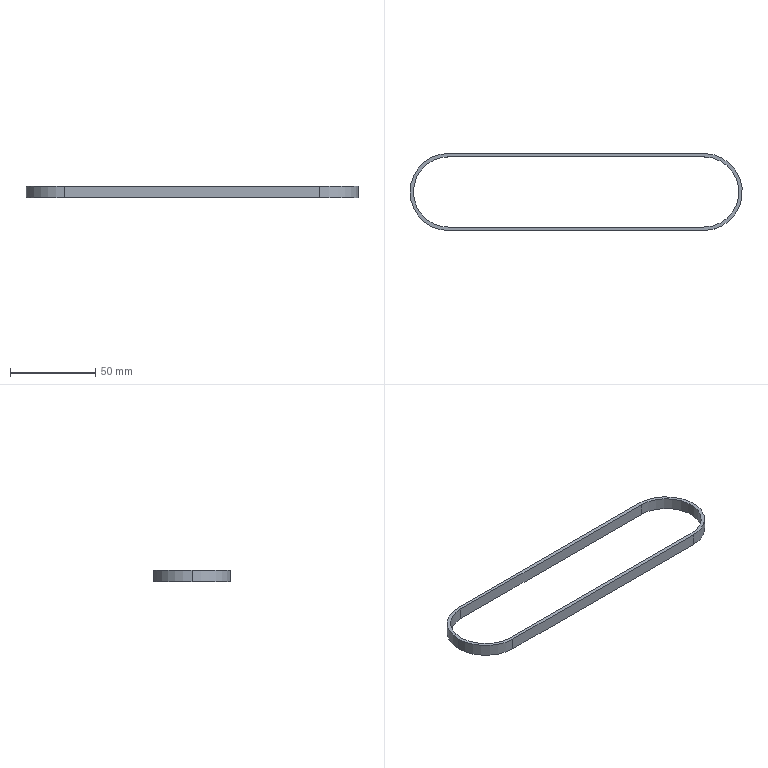Part | SolidWorks | features ExtruThin 1 | 1 solid | 12 faces | box 195.3 x 45.3 x 7 mm | volume 6104 mm3 | cylinder 6 | plane 6 | commonest cylinder face diameters 41.3 x3 45.3 x3
STEP:
#1=CARTESIAN_POINT('',(0.,20.65,3.5));
#2=VERTEX_POINT('',#1);
#3=CARTESIAN_POINT('',(-20.65,0.,3.5));
#4=VERTEX_POINT('',#3);
#5=CARTESIAN_POINT('',(0.,0.,3.5));
#6=DIRECTION('',(0.,0.,1.));
#7=DIRECTION('',(1.,0.,0.));
#8=AXIS2_PLACEMENT_3D('',#5,#6,#7);
#9=CIRCLE('',#8,20.65);
#10=EDGE_CURVE('',#2,#4,#9,.T.);
#11=ORIENTED_EDGE('',*,*,#10,.T.);
#12=CARTESIAN_POINT('',(-20.65,0.,-3.5));
#13=VERTEX_POINT('',#12);
#14=CARTESIAN_POINT('',(-20.65,0.,3.5));
#15=DIRECTION('',(0.,0.,-1.));
#16=VECTOR('',#15,1000.);
#17=LINE('',#14,#16);
#18=EDGE_CURVE('',#4,#13,#17,.T.);
#19=ORIENTED_EDGE('',*,*,#18,.T.);
#20=CARTESIAN_POINT('',(0.,20.65,-3.5));
#21=VERTEX_POINT('',#20);
#22=CARTESIAN_POINT('',(0.,0.,-3.5));
#23=DIRECTION('',(0.,0.,1.));
#24=DIRECTION('',(1.,0.,0.));
#25=AXIS2_PLACEMENT_3D('',#22,#23,#24);
#26=CIRCLE('',#25,20.65);
#27=EDGE_CURVE('',#21,#13,#26,.T.);
#28=ORIENTED_EDGE('',*,*,#27,.F.);
#29=CARTESIAN_POINT('',(0.,20.65,3.5));
#30=DIRECTION('',(0.,0.,-1.));
#31=VECTOR('',#30,1000.);
#32=LINE('',#29,#31);
#33=EDGE_CURVE('',#2,#21,#32,.T.);
#34=ORIENTED_EDGE('',*,*,#33,.F.);
#35=EDGE_LOOP('',(#11,#19,#28,#34));
#36=FACE_OUTER_BOUND('',#35,.T.);
#37=CARTESIAN_POINT('',(0.,0.,3.5));
#38=DIRECTION('',(0.,0.,-1.));
#39=DIRECTION('',(-1.,0.,0.));
#40=AXIS2_PLACEMENT_3D('',#37,#38,#39);
#41=CYLINDRICAL_SURFACE('',#40,20.65);
#42=ADVANCED_FACE('',(#36),#41,.F.);
#43=CARTESIAN_POINT('',(-22.65,0.,3.5));
#44=VERTEX_POINT('',#43);
#45=CARTESIAN_POINT('',(0.,-22.65,3.5));
#46=VERTEX_POINT('',#45);
#47=CARTESIAN_POINT('',(0.,0.,3.5));
#48=DIRECTION('',(0.,0.,1.));
#49=DIRECTION('',(1.,0.,0.));
#50=AXIS2_PLACEMENT_3D('',#47,#48,#49);
#51=CIRCLE('',#50,22.65);
#52=EDGE_CURVE('',#44,#46,#51,.T.);
#53=ORIENTED_EDGE('',*,*,#52,.F.);
#54=CARTESIAN_POINT('',(-22.65,0.,-3.5));
#55=VERTEX_POINT('',#54);
#56=CARTESIAN_POINT('',(-22.65,0.,3.5));
#57=DIRECTION('',(0.,0.,-1.));
#58=VECTOR('',#57,1000.);
#59=LINE('',#56,#58);
#60=EDGE_CURVE('',#44,#55,#59,.T.);
#61=ORIENTED_EDGE('',*,*,#60,.T.);
#62=CARTESIAN_POINT('',(0.,-22.65,-3.5));
#63=VERTEX_POINT('',#62);
#64=CARTESIAN_POINT('',(0.,0.,-3.5));
#65=DIRECTION('',(0.,0.,1.));
#66=DIRECTION('',(1.,0.,0.));
#67=AXIS2_PLACEMENT_3D('',#64,#65,#66);
#68=CIRCLE('',#67,22.65);
#69=EDGE_CURVE('',#55,#63,#68,.T.);
#70=ORIENTED_EDGE('',*,*,#69,.T.);
#71=CARTESIAN_POINT('',(0.,-22.65,3.5));
#72=DIRECTION('',(0.,0.,-1.));
#73=VECTOR('',#72,1000.);
#74=LINE('',#71,#73);
#75=EDGE_CURVE('',#46,#63,#74,.T.);
#76=ORIENTED_EDGE('',*,*,#75,.F.);
#77=EDGE_LOOP('',(#53,#61,#70,#76));
#78=FACE_OUTER_BOUND('',#77,.T.);
#79=CARTESIAN_POINT('',(0.,0.,3.5));
#80=DIRECTION('',(0.,0.,-1.));
#81=DIRECTION('',(-1.,0.,0.));
#82=AXIS2_PLACEMENT_3D('',#79,#80,#81);
#83=CYLINDRICAL_SURFACE('',#82,22.65);
#84=ADVANCED_FACE('',(#78),#83,.T.);
#85=CARTESIAN_POINT('',(0.,22.65,3.5));
#86=VERTEX_POINT('',#85);
#87=CARTESIAN_POINT('',(0.,0.,3.5));
#88=DIRECTION('',(0.,0.,1.));
#89=DIRECTION('',(1.,0.,0.));
#90=AXIS2_PLACEMENT_3D('',#87,#88,#89);
#91=CIRCLE('',#90,22.65);
#92=EDGE_CURVE('',#86,#44,#91,.T.);
#93=ORIENTED_EDGE('',*,*,#92,.T.);
#94=ORIENTED_EDGE('',*,*,#52,.T.);
#95=CARTESIAN_POINT('',(150.,-22.65,3.5));
#96=VERTEX_POINT('',#95);
#97=CARTESIAN_POINT('',(0.,-22.65,3.5));
#98=DIRECTION('',(1.,0.,0.));
#99=VECTOR('',#98,1000.);
#100=LINE('',#97,#99);
#101=EDGE_CURVE('',#46,#96,#100,.T.);
#102=ORIENTED_EDGE('',*,*,#101,.T.);
#103=CARTESIAN_POINT('',(150.,22.65,3.5));
#104=VERTEX_POINT('',#103);
#105=CARTESIAN_POINT('',(150.,0.,3.5));
#106=DIRECTION('',(0.,0.,1.));
#107=DIRECTION('',(1.,0.,0.));
#108=AXIS2_PLACEMENT_3D('',#105,#106,#107);
#109=CIRCLE('',#108,22.65);
#110=EDGE_CURVE('',#96,#104,#109,.T.);
#111=ORIENTED_EDGE('',*,*,#110,.T.);
#112=CARTESIAN_POINT('',(0.,22.65,3.5));
#113=DIRECTION('',(-1.,0.,0.));
#114=VECTOR('',#113,1000.);
#115=LINE('',#112,#114);
#116=EDGE_CURVE('',#104,#86,#115,.T.);
#117=ORIENTED_EDGE('',*,*,#116,.T.);
#118=EDGE_LOOP('',(#93,#94,#102,#111,#117));
#119=FACE_OUTER_BOUND('',#118,.T.);
#120=CARTESIAN_POINT('',(0.,-20.65,3.5));
#121=VERTEX_POINT('',#120);
#122=CARTESIAN_POINT('',(150.,-20.65,3.5));
#123=VERTEX_POINT('',#122);
#124=CARTESIAN_POINT('',(0.,-20.65,3.5));
#125=DIRECTION('',(1.,0.,0.));
#126=VECTOR('',#125,1000.);
#127=LINE('',#124,#126);
#128=EDGE_CURVE('',#121,#123,#127,.T.);
#129=ORIENTED_EDGE('',*,*,#128,.F.);
#130=CARTESIAN_POINT('',(0.,0.,3.5));
#131=DIRECTION('',(0.,0.,1.));
#132=DIRECTION('',(1.,0.,0.));
#133=AXIS2_PLACEMENT_3D('',#130,#131,#132);
#134=CIRCLE('',#133,20.65);
#135=EDGE_CURVE('',#4,#121,#134,.T.);
#136=ORIENTED_EDGE('',*,*,#135,.F.);
#137=ORIENTED_EDGE('',*,*,#10,.F.);
#138=CARTESIAN_POINT('',(150.,20.65,3.5));
#139=VERTEX_POINT('',#138);
#140=CARTESIAN_POINT('',(0.,20.65,3.5));
#141=DIRECTION('',(-1.,0.,0.));
#142=VECTOR('',#141,1000.);
#143=LINE('',#140,#142);
#144=EDGE_CURVE('',#139,#2,#143,.T.);
#145=ORIENTED_EDGE('',*,*,#144,.F.);
#146=CARTESIAN_POINT('',(150.,0.,3.5));
#147=DIRECTION('',(0.,0.,1.));
#148=DIRECTION('',(1.,0.,0.));
#149=AXIS2_PLACEMENT_3D('',#146,#147,#148);
#150=CIRCLE('',#149,20.65);
#151=EDGE_CURVE('',#123,#139,#150,.T.);
#152=ORIENTED_EDGE('',*,*,#151,.F.);
#153=EDGE_LOOP('',(#129,#136,#137,#145,#152));
#154=FACE_BOUND('',#153,.T.);
#155=CARTESIAN_POINT('',(0.,0.,3.5));
#156=DIRECTION('',(0.,0.,1.));
#157=DIRECTION('',(1.,0.,0.));
#158=AXIS2_PLACEMENT_3D('',#155,#156,#157);
#159=PLANE('',#158);
#160=ADVANCED_FACE('',(#119,#154),#159,.T.);
#161=CARTESIAN_POINT('',(0.,22.65,-3.5));
#162=VERTEX_POINT('',#161);
#163=CARTESIAN_POINT('',(0.,0.,-3.5));
#164=DIRECTION('',(0.,0.,1.));
#165=DIRECTION('',(1.,0.,0.));
#166=AXIS2_PLACEMENT_3D('',#163,#164,#165);
#167=CIRCLE('',#166,22.65);
#168=EDGE_CURVE('',#162,#55,#167,.T.);
#169=ORIENTED_EDGE('',*,*,#168,.F.);
#170=CARTESIAN_POINT('',(150.,22.65,-3.5));
#171=VERTEX_POINT('',#170);
#172=CARTESIAN_POINT('',(0.,22.65,-3.5));
#173=DIRECTION('',(-1.,0.,0.));
#174=VECTOR('',#173,1000.);
#175=LINE('',#172,#174);
#176=EDGE_CURVE('',#171,#162,#175,.T.);
#177=ORIENTED_EDGE('',*,*,#176,.F.);
#178=CARTESIAN_POINT('',(150.,-22.65,-3.5));
#179=VERTEX_POINT('',#178);
#180=CARTESIAN_POINT('',(150.,0.,-3.5));
#181=DIRECTION('',(0.,0.,1.));
#182=DIRECTION('',(1.,0.,0.));
#183=AXIS2_PLACEMENT_3D('',#180,#181,#182);
#184=CIRCLE('',#183,22.65);
#185=EDGE_CURVE('',#179,#171,#184,.T.);
#186=ORIENTED_EDGE('',*,*,#185,.F.);
#187=CARTESIAN_POINT('',(0.,-22.65,-3.5));
#188=DIRECTION('',(1.,0.,0.));
#189=VECTOR('',#188,1000.);
#190=LINE('',#187,#189);
#191=EDGE_CURVE('',#63,#179,#190,.T.);
#192=ORIENTED_EDGE('',*,*,#191,.F.);
#193=ORIENTED_EDGE('',*,*,#69,.F.);
#194=EDGE_LOOP('',(#169,#177,#186,#192,#193));
#195=FACE_OUTER_BOUND('',#194,.T.);
#196=ORIENTED_EDGE('',*,*,#27,.T.);
#197=CARTESIAN_POINT('',(0.,-20.65,-3.5));
#198=VERTEX_POINT('',#197);
#199=CARTESIAN_POINT('',(0.,0.,-3.5));
#200=DIRECTION('',(0.,0.,1.));
#201=DIRECTION('',(1.,0.,0.));
#202=AXIS2_PLACEMENT_3D('',#199,#200,#201);
#203=CIRCLE('',#202,20.65);
#204=EDGE_CURVE('',#13,#198,#203,.T.);
#205=ORIENTED_EDGE('',*,*,#204,.T.);
#206=CARTESIAN_POINT('',(150.,-20.65,-3.5));
#207=VERTEX_POINT('',#206);
#208=CARTESIAN_POINT('',(0.,-20.65,-3.5));
#209=DIRECTION('',(1.,0.,0.));
#210=VECTOR('',#209,1000.);
#211=LINE('',#208,#210);
#212=EDGE_CURVE('',#198,#207,#211,.T.);
#213=ORIENTED_EDGE('',*,*,#212,.T.);
#214=CARTESIAN_POINT('',(150.,20.65,-3.5));
#215=VERTEX_POINT('',#214);
#216=CARTESIAN_POINT('',(150.,0.,-3.5));
#217=DIRECTION('',(0.,0.,1.));
#218=DIRECTION('',(1.,0.,0.));
#219=AXIS2_PLACEMENT_3D('',#216,#217,#218);
#220=CIRCLE('',#219,20.65);
#221=EDGE_CURVE('',#207,#215,#220,.T.);
#222=ORIENTED_EDGE('',*,*,#221,.T.);
#223=CARTESIAN_POINT('',(0.,20.65,-3.5));
#224=DIRECTION('',(-1.,0.,0.));
#225=VECTOR('',#224,1000.);
#226=LINE('',#223,#225);
#227=EDGE_CURVE('',#215,#21,#226,.T.);
#228=ORIENTED_EDGE('',*,*,#227,.T.);
#229=EDGE_LOOP('',(#196,#205,#213,#222,#228));
#230=FACE_BOUND('',#229,.T.);
#231=CARTESIAN_POINT('',(0.,0.,-3.5));
#232=DIRECTION('',(0.,0.,1.));
#233=DIRECTION('',(1.,0.,0.));
#234=AXIS2_PLACEMENT_3D('',#231,#232,#233);
#235=PLANE('',#234);
#236=ADVANCED_FACE('',(#195,#230),#235,.F.);
#237=ORIENTED_EDGE('',*,*,#60,.F.);
#238=ORIENTED_EDGE('',*,*,#92,.F.);
#239=CARTESIAN_POINT('',(0.,22.65,3.5));
#240=DIRECTION('',(0.,0.,-1.));
#241=VECTOR('',#240,1000.);
#242=LINE('',#239,#241);
#243=EDGE_CURVE('',#86,#162,#242,.T.);
#244=ORIENTED_EDGE('',*,*,#243,.T.);
#245=ORIENTED_EDGE('',*,*,#168,.T.);
#246=EDGE_LOOP('',(#237,#238,#244,#245));
#247=FACE_OUTER_BOUND('',#246,.T.);
#248=CARTESIAN_POINT('',(0.,0.,3.5));
#249=DIRECTION('',(0.,0.,-1.));
#250=DIRECTION('',(-1.,0.,0.));
#251=AXIS2_PLACEMENT_3D('',#248,#249,#250);
#252=CYLINDRICAL_SURFACE('',#251,22.65);
#253=ADVANCED_FACE('',(#247),#252,.T.);
#254=ORIENTED_EDGE('',*,*,#191,.T.);
#255=CARTESIAN_POINT('',(150.,-22.65,3.5));
#256=DIRECTION('',(0.,0.,-1.));
#257=VECTOR('',#256,1000.);
#258=LINE('',#255,#257);
#259=EDGE_CURVE('',#96,#179,#258,.T.);
#260=ORIENTED_EDGE('',*,*,#259,.F.);
#261=ORIENTED_EDGE('',*,*,#101,.F.);
#262=ORIENTED_EDGE('',*,*,#75,.T.);
#263=EDGE_LOOP('',(#254,#260,#261,#262));
#264=FACE_OUTER_BOUND('',#263,.T.);
#265=CARTESIAN_POINT('',(0.,-22.65,3.5));
#266=DIRECTION('',(0.,1.,0.));
#267=DIRECTION('',(0.,0.,1.));
#268=AXIS2_PLACEMENT_3D('',#265,#266,#267);
#269=PLANE('',#268);
#270=ADVANCED_FACE('',(#264),#269,.F.);
#271=ORIENTED_EDGE('',*,*,#185,.T.);
#272=CARTESIAN_POINT('',(150.,22.65,3.5));
#273=DIRECTION('',(0.,0.,-1.));
#274=VECTOR('',#273,1000.);
#275=LINE('',#272,#274);
#276=EDGE_CURVE('',#104,#171,#275,.T.);
#277=ORIENTED_EDGE('',*,*,#276,.F.);
#278=ORIENTED_EDGE('',*,*,#110,.F.);
#279=ORIENTED_EDGE('',*,*,#259,.T.);
#280=EDGE_LOOP('',(#271,#277,#278,#279));
#281=FACE_OUTER_BOUND('',#280,.T.);
#282=CARTESIAN_POINT('',(150.,0.,3.5));
#283=DIRECTION('',(0.,0.,-1.));
#284=DIRECTION('',(-1.,0.,0.));
#285=AXIS2_PLACEMENT_3D('',#282,#283,#284);
#286=CYLINDRICAL_SURFACE('',#285,22.65);
#287=ADVANCED_FACE('',(#281),#286,.T.);
#288=ORIENTED_EDGE('',*,*,#176,.T.);
#289=ORIENTED_EDGE('',*,*,#243,.F.);
#290=ORIENTED_EDGE('',*,*,#116,.F.);
#291=ORIENTED_EDGE('',*,*,#276,.T.);
#292=EDGE_LOOP('',(#288,#289,#290,#291));
#293=FACE_OUTER_BOUND('',#292,.T.);
#294=CARTESIAN_POINT('',(0.,22.65,3.5));
#295=DIRECTION('',(0.,-1.,0.));
#296=DIRECTION('',(0.,0.,-1.));
#297=AXIS2_PLACEMENT_3D('',#294,#295,#296);
#298=PLANE('',#297);
#299=ADVANCED_FACE('',(#293),#298,.F.);
#300=ORIENTED_EDGE('',*,*,#18,.F.);
#301=ORIENTED_EDGE('',*,*,#135,.T.);
#302=CARTESIAN_POINT('',(0.,-20.65,3.5));
#303=DIRECTION('',(0.,0.,-1.));
#304=VECTOR('',#303,1000.);
#305=LINE('',#302,#304);
#306=EDGE_CURVE('',#121,#198,#305,.T.);
#307=ORIENTED_EDGE('',*,*,#306,.T.);
#308=ORIENTED_EDGE('',*,*,#204,.F.);
#309=EDGE_LOOP('',(#300,#301,#307,#308));
#310=FACE_OUTER_BOUND('',#309,.T.);
#311=CARTESIAN_POINT('',(0.,0.,3.5));
#312=DIRECTION('',(0.,0.,-1.));
#313=DIRECTION('',(-1.,0.,0.));
#314=AXIS2_PLACEMENT_3D('',#311,#312,#313);
#315=CYLINDRICAL_SURFACE('',#314,20.65);
#316=ADVANCED_FACE('',(#310),#315,.F.);
#317=ORIENTED_EDGE('',*,*,#212,.F.);
#318=ORIENTED_EDGE('',*,*,#306,.F.);
#319=ORIENTED_EDGE('',*,*,#128,.T.);
#320=CARTESIAN_POINT('',(150.,-20.65,3.5));
#321=DIRECTION('',(0.,0.,-1.));
#322=VECTOR('',#321,1000.);
#323=LINE('',#320,#322);
#324=EDGE_CURVE('',#123,#207,#323,.T.);
#325=ORIENTED_EDGE('',*,*,#324,.T.);
#326=EDGE_LOOP('',(#317,#318,#319,#325));
#327=FACE_OUTER_BOUND('',#326,.T.);
#328=CARTESIAN_POINT('',(0.,-20.65,3.5));
#329=DIRECTION('',(0.,1.,0.));
#330=DIRECTION('',(0.,0.,1.));
#331=AXIS2_PLACEMENT_3D('',#328,#329,#330);
#332=PLANE('',#331);
#333=ADVANCED_FACE('',(#327),#332,.T.);
#334=ORIENTED_EDGE('',*,*,#221,.F.);
#335=ORIENTED_EDGE('',*,*,#324,.F.);
#336=ORIENTED_EDGE('',*,*,#151,.T.);
#337=CARTESIAN_POINT('',(150.,20.65,3.5));
#338=DIRECTION('',(0.,0.,-1.));
#339=VECTOR('',#338,1000.);
#340=LINE('',#337,#339);
#341=EDGE_CURVE('',#139,#215,#340,.T.);
#342=ORIENTED_EDGE('',*,*,#341,.T.);
#343=EDGE_LOOP('',(#334,#335,#336,#342));
#344=FACE_OUTER_BOUND('',#343,.T.);
#345=CARTESIAN_POINT('',(150.,0.,3.5));
#346=DIRECTION('',(0.,0.,-1.));
#347=DIRECTION('',(-1.,0.,0.));
#348=AXIS2_PLACEMENT_3D('',#345,#346,#347);
#349=CYLINDRICAL_SURFACE('',#348,20.65);
#350=ADVANCED_FACE('',(#344),#349,.F.);
#351=ORIENTED_EDGE('',*,*,#227,.F.);
#352=ORIENTED_EDGE('',*,*,#341,.F.);
#353=ORIENTED_EDGE('',*,*,#144,.T.);
#354=ORIENTED_EDGE('',*,*,#33,.T.);
#355=EDGE_LOOP('',(#351,#352,#353,#354));
#356=FACE_OUTER_BOUND('',#355,.T.);
#357=CARTESIAN_POINT('',(0.,20.65,3.5));
#358=DIRECTION('',(0.,-1.,0.));
#359=DIRECTION('',(0.,0.,-1.));
#360=AXIS2_PLACEMENT_3D('',#357,#358,#359);
#361=PLANE('',#360);
#362=ADVANCED_FACE('',(#356),#361,.T.);
#363=CLOSED_SHELL('',(#42,#84,#160,#236,#253,#270,#287,#299,#316,#333,#350,#362));
#364=MANIFOLD_SOLID_BREP('',#363);
#365=CARTESIAN_POINT('',(0.,0.,0.));
#366=DIRECTION('',(0.,0.,1.));
#367=DIRECTION('',(1.,0.,0.));
#368=AXIS2_PLACEMENT_3D('',#365,#366,#367);
#369=(LENGTH_UNIT()NAMED_UNIT(*)SI_UNIT(.MILLI.,.METRE.));
#370=UNCERTAINTY_MEASURE_WITH_UNIT(LENGTH_MEASURE(0.00001),#369,'','');
#371=(NAMED_UNIT(*)PLANE_ANGLE_UNIT()SI_UNIT($,.RADIAN.));
#372=(NAMED_UNIT(*)SI_UNIT($,.STERADIAN.)SOLID_ANGLE_UNIT());
#373=(GEOMETRIC_REPRESENTATION_CONTEXT(3)GLOBAL_UNCERTAINTY_ASSIGNED_CONTEXT((#370))GLOBAL_UNIT_ASSIGNED_CONTEXT((#369,#371,#372))REPRESENTATION_CONTEXT('',''));
#374=ADVANCED_BREP_SHAPE_REPRESENTATION('',(#364,#368),#373);